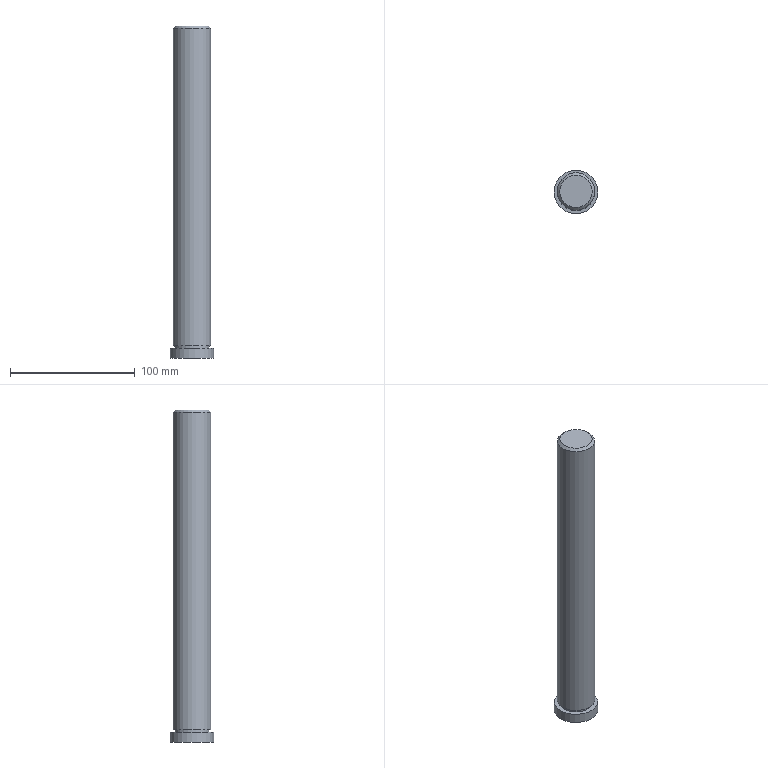Part | STEP file | 车灯-后视镜_id82_x_t | 1 solid | 8 faces | box 35 x 35 x 266 mm | volume 189704 mm3 | plane 4 | cylinder 3 | cone 1 | commonest cylinder face diameters 28 x1 30 x1 35 x1
STEP:
#1=CARTESIAN_POINT('',(140.5,-242.,-265.5));
#2=VERTEX_POINT('',#1);
#3=CARTESIAN_POINT('',(123.,-242.,-265.5));
#4=DIRECTION('',(0.,0.,-1.));
#5=DIRECTION('',(1.,0.,0.));
#6=AXIS2_PLACEMENT_3D('',#3,#4,#5);
#7=CIRCLE('',#6,17.5);
#8=EDGE_CURVE('',#2,#2,#7,.T.);
#9=ORIENTED_EDGE('',*,*,#8,.T.);
#10=EDGE_LOOP('',(#9));
#11=FACE_OUTER_BOUND('',#10,.T.);
#12=CARTESIAN_POINT('',(123.,-242.,-265.5));
#13=DIRECTION('',(0.,0.,-1.));
#14=DIRECTION('',(-1.,0.,0.));
#15=AXIS2_PLACEMENT_3D('',#12,#13,#14);
#16=PLANE('',#15);
#17=ADVANCED_FACE('',(#11),#16,.T.);
#18=CARTESIAN_POINT('',(105.5,-242.,-257.5));
#19=VERTEX_POINT('',#18);
#20=CARTESIAN_POINT('',(123.,-242.,-257.5));
#21=DIRECTION('',(0.,0.,1.));
#22=DIRECTION('',(-1.,0.,0.));
#23=AXIS2_PLACEMENT_3D('',#20,#21,#22);
#24=CIRCLE('',#23,17.5);
#25=EDGE_CURVE('',#19,#19,#24,.T.);
#26=ORIENTED_EDGE('',*,*,#25,.T.);
#27=EDGE_LOOP('',(#26));
#28=FACE_BOUND('',#27,.T.);
#29=CARTESIAN_POINT('',(137.,-242.,-257.5));
#30=VERTEX_POINT('',#29);
#31=CARTESIAN_POINT('',(123.,-242.,-257.5));
#32=DIRECTION('',(0.,0.,-1.));
#33=DIRECTION('',(1.,0.,0.));
#34=AXIS2_PLACEMENT_3D('',#31,#32,#33);
#35=CIRCLE('',#34,14.);
#36=EDGE_CURVE('',#30,#30,#35,.T.);
#37=ORIENTED_EDGE('',*,*,#36,.T.);
#38=EDGE_LOOP('',(#37));
#39=FACE_BOUND('',#38,.T.);
#40=CARTESIAN_POINT('',(123.,-242.,-257.5));
#41=DIRECTION('',(0.,0.,1.));
#42=DIRECTION('',(1.,0.,0.));
#43=AXIS2_PLACEMENT_3D('',#40,#41,#42);
#44=PLANE('',#43);
#45=ADVANCED_FACE('',(#28,#39),#44,.T.);
#46=ORIENTED_EDGE('',*,*,#8,.F.);
#47=EDGE_LOOP('',(#46));
#48=FACE_BOUND('',#47,.T.);
#49=ORIENTED_EDGE('',*,*,#25,.F.);
#50=EDGE_LOOP('',(#49));
#51=FACE_BOUND('',#50,.T.);
#52=CARTESIAN_POINT('',(123.,-242.,-257.5));
#53=DIRECTION('',(0.,0.,-1.));
#54=DIRECTION('',(-1.,0.,0.));
#55=AXIS2_PLACEMENT_3D('',#52,#53,#54);
#56=CYLINDRICAL_SURFACE('',#55,17.5);
#57=ADVANCED_FACE('',(#48,#51),#56,.T.);
#58=CARTESIAN_POINT('',(137.,-242.,-255.5));
#59=VERTEX_POINT('',#58);
#60=CARTESIAN_POINT('',(123.,-242.,-255.5));
#61=DIRECTION('',(0.,0.,-1.));
#62=DIRECTION('',(1.,0.,0.));
#63=AXIS2_PLACEMENT_3D('',#60,#61,#62);
#64=CIRCLE('',#63,14.);
#65=EDGE_CURVE('',#59,#59,#64,.T.);
#66=ORIENTED_EDGE('',*,*,#65,.T.);
#67=EDGE_LOOP('',(#66));
#68=FACE_BOUND('',#67,.T.);
#69=ORIENTED_EDGE('',*,*,#36,.F.);
#70=EDGE_LOOP('',(#69));
#71=FACE_BOUND('',#70,.T.);
#72=CARTESIAN_POINT('',(123.,-242.,-256.5));
#73=DIRECTION('',(0.,0.,1.));
#74=DIRECTION('',(1.,0.,0.));
#75=AXIS2_PLACEMENT_3D('',#72,#73,#74);
#76=CYLINDRICAL_SURFACE('',#75,14.);
#77=ADVANCED_FACE('',(#68,#71),#76,.T.);
#78=CARTESIAN_POINT('',(138.,-242.,-255.5));
#79=VERTEX_POINT('',#78);
#80=CARTESIAN_POINT('',(123.,-242.,-255.5));
#81=DIRECTION('',(0.,0.,1.));
#82=DIRECTION('',(1.,0.,0.));
#83=AXIS2_PLACEMENT_3D('',#80,#81,#82);
#84=CIRCLE('',#83,15.);
#85=EDGE_CURVE('',#79,#79,#84,.T.);
#86=ORIENTED_EDGE('',*,*,#85,.F.);
#87=EDGE_LOOP('',(#86));
#88=FACE_BOUND('',#87,.T.);
#89=ORIENTED_EDGE('',*,*,#65,.F.);
#90=EDGE_LOOP('',(#89));
#91=FACE_BOUND('',#90,.T.);
#92=CARTESIAN_POINT('',(123.,-242.,-255.5));
#93=DIRECTION('',(0.,0.,1.));
#94=DIRECTION('',(1.,0.,0.));
#95=AXIS2_PLACEMENT_3D('',#92,#93,#94);
#96=PLANE('',#95);
#97=ADVANCED_FACE('',(#88,#91),#96,.F.);
#98=CARTESIAN_POINT('',(136.,-242.,0.5));
#99=VERTEX_POINT('',#98);
#100=CARTESIAN_POINT('',(123.,-242.,0.5));
#101=DIRECTION('',(0.,0.,-1.));
#102=DIRECTION('',(1.,0.,0.));
#103=AXIS2_PLACEMENT_3D('',#100,#101,#102);
#104=CIRCLE('',#103,13.);
#105=EDGE_CURVE('',#99,#99,#104,.T.);
#106=ORIENTED_EDGE('',*,*,#105,.F.);
#107=EDGE_LOOP('',(#106));
#108=FACE_OUTER_BOUND('',#107,.T.);
#109=CARTESIAN_POINT('',(123.,-242.,0.5));
#110=DIRECTION('',(0.,0.,1.));
#111=DIRECTION('',(1.,0.,0.));
#112=AXIS2_PLACEMENT_3D('',#109,#110,#111);
#113=PLANE('',#112);
#114=ADVANCED_FACE('',(#108),#113,.T.);
#115=CARTESIAN_POINT('',(138.,-242.,-1.5));
#116=VERTEX_POINT('',#115);
#117=CARTESIAN_POINT('',(123.,-242.,-1.5));
#118=DIRECTION('',(0.,0.,1.));
#119=DIRECTION('',(1.,0.,0.));
#120=AXIS2_PLACEMENT_3D('',#117,#118,#119);
#121=CIRCLE('',#120,15.);
#122=EDGE_CURVE('',#116,#116,#121,.T.);
#123=ORIENTED_EDGE('',*,*,#122,.F.);
#124=EDGE_LOOP('',(#123));
#125=FACE_BOUND('',#124,.T.);
#126=ORIENTED_EDGE('',*,*,#85,.T.);
#127=EDGE_LOOP('',(#126));
#128=FACE_BOUND('',#127,.T.);
#129=CARTESIAN_POINT('',(123.,-242.,-135.));
#130=DIRECTION('',(0.,0.,1.));
#131=DIRECTION('',(1.,0.,0.));
#132=AXIS2_PLACEMENT_3D('',#129,#130,#131);
#133=CYLINDRICAL_SURFACE('',#132,15.);
#134=ADVANCED_FACE('',(#125,#128),#133,.T.);
#135=ORIENTED_EDGE('',*,*,#105,.T.);
#136=EDGE_LOOP('',(#135));
#137=FACE_BOUND('',#136,.T.);
#138=ORIENTED_EDGE('',*,*,#122,.T.);
#139=EDGE_LOOP('',(#138));
#140=FACE_BOUND('',#139,.T.);
#141=CARTESIAN_POINT('',(123.,-242.,-1.5));
#142=DIRECTION('',(0.,0.,-1.));
#143=DIRECTION('',(-1.,0.,0.));
#144=AXIS2_PLACEMENT_3D('',#141,#142,#143);
#145=CONICAL_SURFACE('',#144,15.,45.);
#146=ADVANCED_FACE('',(#137,#140),#145,.T.);
#147=CLOSED_SHELL('',(#17,#45,#57,#77,#97,#114,#134,#146));
#148=MANIFOLD_SOLID_BREP('',#147);
#149=(LENGTH_UNIT()NAMED_UNIT(*)SI_UNIT(.MILLI.,.METRE.));
#150=UNCERTAINTY_MEASURE_WITH_UNIT(LENGTH_MEASURE(0.00002),#149,'','');
#151=(NAMED_UNIT(*)PLANE_ANGLE_UNIT()SI_UNIT($,.RADIAN.));
#152=PLANE_ANGLE_MEASURE_WITH_UNIT(PLANE_ANGLE_MEASURE(0.01745),#151);
#153=DIMENSIONAL_EXPONENTS(0.,0.,0.,0.,0.,0.,0.);
#154=(CONVERSION_BASED_UNIT('DEGREE',#152)NAMED_UNIT(#153)PLANE_ANGLE_UNIT());
#155=(NAMED_UNIT(*)SI_UNIT($,.STERADIAN.)SOLID_ANGLE_UNIT());
#156=(GEOMETRIC_REPRESENTATION_CONTEXT(3)GLOBAL_UNCERTAINTY_ASSIGNED_CONTEXT((#150))GLOBAL_UNIT_ASSIGNED_CONTEXT((#149,#154,#155))REPRESENTATION_CONTEXT('',''));
#157=ADVANCED_BREP_SHAPE_REPRESENTATION('',(#148),#156);